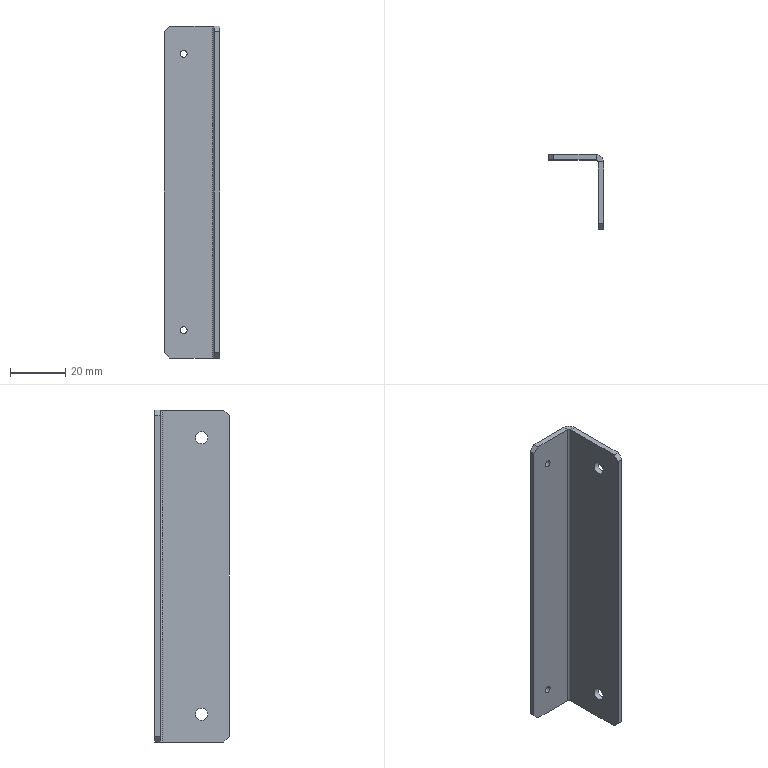Part | NX | 1 solid | 22 faces | box 20 x 27 x 120 mm | volume 10522 mm3 | plane 16 | cylinder 6 | commonest cylinder face diameters 2.5 x2 4.5 x2 1.473 x1 5.473 x1
STEP:
#1=CARTESIAN_POINT('',(-7.,0.,60.));
#2=VERTEX_POINT('',#1);
#3=CARTESIAN_POINT('',(8.263,0.,60.));
#4=VERTEX_POINT('',#3);
#5=CARTESIAN_POINT('',(-9.,0.,60.));
#6=DIRECTION('',(1.,0.,0.));
#7=VECTOR('',#6,1000.);
#8=LINE('',#5,#7);
#9=EDGE_CURVE('',#2,#4,#8,.T.);
#10=ORIENTED_EDGE('',*,*,#9,.F.);
#11=CARTESIAN_POINT('',(-7.,-2.,60.));
#12=VERTEX_POINT('',#11);
#13=CARTESIAN_POINT('',(-7.,-2.,60.));
#14=DIRECTION('',(0.,-1.,0.));
#15=VECTOR('',#14,1000.);
#16=LINE('',#13,#15);
#17=EDGE_CURVE('',#2,#12,#16,.T.);
#18=ORIENTED_EDGE('',*,*,#17,.T.);
#19=CARTESIAN_POINT('',(8.263,-2.,60.));
#20=VERTEX_POINT('',#19);
#21=CARTESIAN_POINT('',(-9.,-2.,60.));
#22=DIRECTION('',(1.,0.,0.));
#23=VECTOR('',#22,1000.);
#24=LINE('',#21,#23);
#25=EDGE_CURVE('',#12,#20,#24,.T.);
#26=ORIENTED_EDGE('',*,*,#25,.T.);
#27=CARTESIAN_POINT('',(8.263,-2.,60.));
#28=DIRECTION('',(0.,1.,0.));
#29=VECTOR('',#28,1000.);
#30=LINE('',#27,#29);
#31=EDGE_CURVE('',#20,#4,#30,.T.);
#32=ORIENTED_EDGE('',*,*,#31,.T.);
#33=EDGE_LOOP('',(#10,#18,#26,#32));
#34=FACE_BOUND('',#33,.T.);
#35=CARTESIAN_POINT('',(-9.,-2.,60.));
#36=DIRECTION('',(0.,0.,1.));
#37=DIRECTION('',(1.,0.,0.));
#38=AXIS2_PLACEMENT_3D('',#35,#36,#37);
#39=PLANE('',#38);
#40=ADVANCED_FACE('',(#34),#39,.T.);
#41=CARTESIAN_POINT('',(-2.,-2.,-51.25));
#42=VERTEX_POINT('',#41);
#43=CARTESIAN_POINT('',(-2.,-2.,-50.));
#44=DIRECTION('',(0.,-1.,0.));
#45=DIRECTION('',(0.,0.,-1.));
#46=AXIS2_PLACEMENT_3D('',#43,#44,#45);
#47=CIRCLE('',#46,1.25);
#48=EDGE_CURVE('',#42,#42,#47,.T.);
#49=ORIENTED_EDGE('',*,*,#48,.F.);
#50=EDGE_LOOP('',(#49));
#51=FACE_BOUND('',#50,.T.);
#52=CARTESIAN_POINT('',(-2.,-2.,48.75));
#53=VERTEX_POINT('',#52);
#54=CARTESIAN_POINT('',(-2.,-2.,50.));
#55=DIRECTION('',(0.,-1.,0.));
#56=DIRECTION('',(0.,0.,-1.));
#57=AXIS2_PLACEMENT_3D('',#54,#55,#56);
#58=CIRCLE('',#57,1.25);
#59=EDGE_CURVE('',#53,#53,#58,.T.);
#60=ORIENTED_EDGE('',*,*,#59,.F.);
#61=EDGE_LOOP('',(#60));
#62=FACE_BOUND('',#61,.T.);
#63=ORIENTED_EDGE('',*,*,#25,.F.);
#64=CARTESIAN_POINT('',(-9.,-2.,58.));
#65=VERTEX_POINT('',#64);
#66=CARTESIAN_POINT('',(-33.5,-2.,33.5));
#67=DIRECTION('',(0.7071,0.,0.7071));
#68=VECTOR('',#67,1000.);
#69=LINE('',#66,#68);
#70=EDGE_CURVE('',#12,#65,#69,.F.);
#71=ORIENTED_EDGE('',*,*,#70,.T.);
#72=CARTESIAN_POINT('',(-9.,-2.,-58.));
#73=VERTEX_POINT('',#72);
#74=CARTESIAN_POINT('',(-9.,-2.,60.));
#75=DIRECTION('',(0.,0.,1.));
#76=VECTOR('',#75,1000.);
#77=LINE('',#74,#76);
#78=EDGE_CURVE('',#73,#65,#77,.T.);
#79=ORIENTED_EDGE('',*,*,#78,.F.);
#80=CARTESIAN_POINT('',(-7.,-2.,-60.));
#81=VERTEX_POINT('',#80);
#82=CARTESIAN_POINT('',(-33.5,-2.,-33.5));
#83=DIRECTION('',(-0.7071,0.,0.7071));
#84=VECTOR('',#83,1000.);
#85=LINE('',#82,#84);
#86=EDGE_CURVE('',#73,#81,#85,.F.);
#87=ORIENTED_EDGE('',*,*,#86,.T.);
#88=CARTESIAN_POINT('',(8.263,-2.,-60.));
#89=VERTEX_POINT('',#88);
#90=CARTESIAN_POINT('',(-9.,-2.,-60.));
#91=DIRECTION('',(-1.,0.,0.));
#92=VECTOR('',#91,1000.);
#93=LINE('',#90,#92);
#94=EDGE_CURVE('',#89,#81,#93,.T.);
#95=ORIENTED_EDGE('',*,*,#94,.F.);
#96=CARTESIAN_POINT('',(8.263,-2.,60.));
#97=DIRECTION('',(0.,0.,1.));
#98=VECTOR('',#97,1000.);
#99=LINE('',#96,#98);
#100=EDGE_CURVE('',#20,#89,#99,.F.);
#101=ORIENTED_EDGE('',*,*,#100,.F.);
#102=EDGE_LOOP('',(#63,#71,#79,#87,#95,#101));
#103=FACE_BOUND('',#102,.T.);
#104=CARTESIAN_POINT('',(0.,-2.,0.));
#105=DIRECTION('',(0.,-1.,0.));
#106=DIRECTION('',(0.,0.,-1.));
#107=AXIS2_PLACEMENT_3D('',#104,#105,#106);
#108=PLANE('',#107);
#109=ADVANCED_FACE('',(#51,#62,#103),#108,.T.);
#110=CARTESIAN_POINT('',(-2.,0.,-48.75));
#111=VERTEX_POINT('',#110);
#112=CARTESIAN_POINT('',(-2.,0.,-50.));
#113=DIRECTION('',(0.,1.,0.));
#114=DIRECTION('',(0.,0.,1.));
#115=AXIS2_PLACEMENT_3D('',#112,#113,#114);
#116=CIRCLE('',#115,1.25);
#117=EDGE_CURVE('',#111,#111,#116,.T.);
#118=ORIENTED_EDGE('',*,*,#117,.F.);
#119=EDGE_LOOP('',(#118));
#120=FACE_BOUND('',#119,.T.);
#121=CARTESIAN_POINT('',(-2.,0.,51.25));
#122=VERTEX_POINT('',#121);
#123=CARTESIAN_POINT('',(-2.,0.,50.));
#124=DIRECTION('',(0.,1.,0.));
#125=DIRECTION('',(0.,0.,1.));
#126=AXIS2_PLACEMENT_3D('',#123,#124,#125);
#127=CIRCLE('',#126,1.25);
#128=EDGE_CURVE('',#122,#122,#127,.T.);
#129=ORIENTED_EDGE('',*,*,#128,.F.);
#130=EDGE_LOOP('',(#129));
#131=FACE_BOUND('',#130,.T.);
#132=CARTESIAN_POINT('',(-9.,0.,-58.));
#133=VERTEX_POINT('',#132);
#134=CARTESIAN_POINT('',(-9.,0.,58.));
#135=VERTEX_POINT('',#134);
#136=CARTESIAN_POINT('',(-9.,0.,60.));
#137=DIRECTION('',(0.,0.,1.));
#138=VECTOR('',#137,1000.);
#139=LINE('',#136,#138);
#140=EDGE_CURVE('',#133,#135,#139,.T.);
#141=ORIENTED_EDGE('',*,*,#140,.T.);
#142=CARTESIAN_POINT('',(-9.,0.,58.));
#143=DIRECTION('',(-0.7071,0.,-0.7071));
#144=VECTOR('',#143,1000.);
#145=LINE('',#142,#144);
#146=EDGE_CURVE('',#135,#2,#145,.F.);
#147=ORIENTED_EDGE('',*,*,#146,.T.);
#148=ORIENTED_EDGE('',*,*,#9,.T.);
#149=CARTESIAN_POINT('',(8.263,0.,-60.));
#150=VERTEX_POINT('',#149);
#151=CARTESIAN_POINT('',(8.263,0.,60.));
#152=DIRECTION('',(0.,0.,1.));
#153=VECTOR('',#152,1000.);
#154=LINE('',#151,#153);
#155=EDGE_CURVE('',#4,#150,#154,.F.);
#156=ORIENTED_EDGE('',*,*,#155,.T.);
#157=CARTESIAN_POINT('',(-7.,0.,-60.));
#158=VERTEX_POINT('',#157);
#159=CARTESIAN_POINT('',(-9.,0.,-60.));
#160=DIRECTION('',(-1.,0.,0.));
#161=VECTOR('',#160,1000.);
#162=LINE('',#159,#161);
#163=EDGE_CURVE('',#150,#158,#162,.T.);
#164=ORIENTED_EDGE('',*,*,#163,.T.);
#165=CARTESIAN_POINT('',(-7.,0.,-60.));
#166=DIRECTION('',(0.7071,0.,-0.7071));
#167=VECTOR('',#166,1000.);
#168=LINE('',#165,#167);
#169=EDGE_CURVE('',#158,#133,#168,.F.);
#170=ORIENTED_EDGE('',*,*,#169,.T.);
#171=EDGE_LOOP('',(#141,#147,#148,#156,#164,#170));
#172=FACE_BOUND('',#171,.T.);
#173=CARTESIAN_POINT('',(0.,0.,0.));
#174=DIRECTION('',(0.,-1.,0.));
#175=DIRECTION('',(0.,0.,-1.));
#176=AXIS2_PLACEMENT_3D('',#173,#174,#175);
#177=PLANE('',#176);
#178=ADVANCED_FACE('',(#120,#131,#172),#177,.F.);
#179=ORIENTED_EDGE('',*,*,#78,.T.);
#180=CARTESIAN_POINT('',(-9.,-2.,58.));
#181=DIRECTION('',(0.,1.,0.));
#182=VECTOR('',#181,1000.);
#183=LINE('',#180,#182);
#184=EDGE_CURVE('',#65,#135,#183,.T.);
#185=ORIENTED_EDGE('',*,*,#184,.T.);
#186=ORIENTED_EDGE('',*,*,#140,.F.);
#187=CARTESIAN_POINT('',(-9.,-2.,-58.));
#188=DIRECTION('',(0.,-1.,0.));
#189=VECTOR('',#188,1000.);
#190=LINE('',#187,#189);
#191=EDGE_CURVE('',#133,#73,#190,.T.);
#192=ORIENTED_EDGE('',*,*,#191,.T.);
#193=EDGE_LOOP('',(#179,#185,#186,#192));
#194=FACE_BOUND('',#193,.T.);
#195=CARTESIAN_POINT('',(-9.,-2.,60.));
#196=DIRECTION('',(-1.,0.,0.));
#197=DIRECTION('',(0.,0.,1.));
#198=AXIS2_PLACEMENT_3D('',#195,#196,#197);
#199=PLANE('',#198);
#200=ADVANCED_FACE('',(#194),#199,.T.);
#201=ORIENTED_EDGE('',*,*,#94,.T.);
#202=CARTESIAN_POINT('',(-7.,-2.,-60.));
#203=DIRECTION('',(0.,1.,0.));
#204=VECTOR('',#203,1000.);
#205=LINE('',#202,#204);
#206=EDGE_CURVE('',#81,#158,#205,.T.);
#207=ORIENTED_EDGE('',*,*,#206,.T.);
#208=ORIENTED_EDGE('',*,*,#163,.F.);
#209=CARTESIAN_POINT('',(8.263,-2.,-60.));
#210=DIRECTION('',(0.,1.,0.));
#211=VECTOR('',#210,1000.);
#212=LINE('',#209,#211);
#213=EDGE_CURVE('',#89,#150,#212,.T.);
#214=ORIENTED_EDGE('',*,*,#213,.F.);
#215=EDGE_LOOP('',(#201,#207,#208,#214));
#216=FACE_BOUND('',#215,.T.);
#217=CARTESIAN_POINT('',(-9.,-2.,-60.));
#218=DIRECTION('',(0.,0.,-1.));
#219=DIRECTION('',(-1.,0.,0.));
#220=AXIS2_PLACEMENT_3D('',#217,#218,#219);
#221=PLANE('',#220);
#222=ADVANCED_FACE('',(#216),#221,.T.);
#223=CARTESIAN_POINT('',(9.,-2.737,-60.));
#224=VERTEX_POINT('',#223);
#225=CARTESIAN_POINT('',(11.,-2.737,-60.));
#226=VERTEX_POINT('',#225);
#227=CARTESIAN_POINT('',(9.,-2.737,-60.));
#228=DIRECTION('',(1.,0.,0.));
#229=VECTOR('',#228,1000.);
#230=LINE('',#227,#229);
#231=EDGE_CURVE('',#224,#226,#230,.T.);
#232=ORIENTED_EDGE('',*,*,#231,.F.);
#233=CARTESIAN_POINT('',(8.263,-2.737,-60.));
#234=DIRECTION('',(0.,0.,1.));
#235=DIRECTION('',(1.,0.,0.));
#236=AXIS2_PLACEMENT_3D('',#233,#234,#235);
#237=CIRCLE('',#236,0.7366);
#238=EDGE_CURVE('',#89,#224,#237,.F.);
#239=ORIENTED_EDGE('',*,*,#238,.F.);
#240=ORIENTED_EDGE('',*,*,#213,.T.);
#241=CARTESIAN_POINT('',(8.263,-2.737,-60.));
#242=DIRECTION('',(0.,0.,1.));
#243=DIRECTION('',(1.,0.,0.));
#244=AXIS2_PLACEMENT_3D('',#241,#242,#243);
#245=CIRCLE('',#244,2.737);
#246=EDGE_CURVE('',#150,#226,#245,.F.);
#247=ORIENTED_EDGE('',*,*,#246,.T.);
#248=EDGE_LOOP('',(#232,#239,#240,#247));
#249=FACE_BOUND('',#248,.T.);
#250=CARTESIAN_POINT('',(8.263,-2.737,-60.));
#251=DIRECTION('',(0.,0.,-1.));
#252=DIRECTION('',(-1.,0.,0.));
#253=AXIS2_PLACEMENT_3D('',#250,#251,#252);
#254=PLANE('',#253);
#255=ADVANCED_FACE('',(#249),#254,.T.);
#256=CARTESIAN_POINT('',(9.,-2.737,60.));
#257=VERTEX_POINT('',#256);
#258=CARTESIAN_POINT('',(8.263,-2.737,60.));
#259=DIRECTION('',(0.,0.,1.));
#260=DIRECTION('',(1.,0.,0.));
#261=AXIS2_PLACEMENT_3D('',#258,#259,#260);
#262=CIRCLE('',#261,0.7366);
#263=EDGE_CURVE('',#257,#20,#262,.T.);
#264=ORIENTED_EDGE('',*,*,#263,.F.);
#265=CARTESIAN_POINT('',(11.,-2.737,60.));
#266=VERTEX_POINT('',#265);
#267=CARTESIAN_POINT('',(9.,-2.737,60.));
#268=DIRECTION('',(1.,0.,0.));
#269=VECTOR('',#268,1000.);
#270=LINE('',#267,#269);
#271=EDGE_CURVE('',#257,#266,#270,.T.);
#272=ORIENTED_EDGE('',*,*,#271,.T.);
#273=CARTESIAN_POINT('',(8.263,-2.737,60.));
#274=DIRECTION('',(0.,0.,1.));
#275=DIRECTION('',(1.,0.,0.));
#276=AXIS2_PLACEMENT_3D('',#273,#274,#275);
#277=CIRCLE('',#276,2.737);
#278=EDGE_CURVE('',#266,#4,#277,.T.);
#279=ORIENTED_EDGE('',*,*,#278,.T.);
#280=ORIENTED_EDGE('',*,*,#31,.F.);
#281=EDGE_LOOP('',(#264,#272,#279,#280));
#282=FACE_BOUND('',#281,.T.);
#283=CARTESIAN_POINT('',(8.263,-2.737,60.));
#284=DIRECTION('',(0.,0.,-1.));
#285=DIRECTION('',(-1.,0.,0.));
#286=AXIS2_PLACEMENT_3D('',#283,#284,#285);
#287=PLANE('',#286);
#288=ADVANCED_FACE('',(#282),#287,.F.);
#289=ORIENTED_EDGE('',*,*,#155,.F.);
#290=ORIENTED_EDGE('',*,*,#278,.F.);
#291=CARTESIAN_POINT('',(11.,-2.737,0.));
#292=DIRECTION('',(0.,0.,1.));
#293=VECTOR('',#292,1000.);
#294=LINE('',#291,#293);
#295=EDGE_CURVE('',#226,#266,#294,.T.);
#296=ORIENTED_EDGE('',*,*,#295,.F.);
#297=ORIENTED_EDGE('',*,*,#246,.F.);
#298=EDGE_LOOP('',(#289,#290,#296,#297));
#299=FACE_BOUND('',#298,.T.);
#300=CARTESIAN_POINT('',(8.263,-2.737,60.));
#301=DIRECTION('',(0.,0.,1.));
#302=DIRECTION('',(1.,0.,0.));
#303=AXIS2_PLACEMENT_3D('',#300,#301,#302);
#304=CYLINDRICAL_SURFACE('',#303,2.737);
#305=ADVANCED_FACE('',(#299),#304,.T.);
#306=ORIENTED_EDGE('',*,*,#100,.T.);
#307=ORIENTED_EDGE('',*,*,#238,.T.);
#308=CARTESIAN_POINT('',(9.,-2.737,-60.));
#309=DIRECTION('',(0.,0.,1.));
#310=VECTOR('',#309,1000.);
#311=LINE('',#308,#310);
#312=EDGE_CURVE('',#224,#257,#311,.T.);
#313=ORIENTED_EDGE('',*,*,#312,.T.);
#314=ORIENTED_EDGE('',*,*,#263,.T.);
#315=EDGE_LOOP('',(#306,#307,#313,#314));
#316=FACE_BOUND('',#315,.T.);
#317=CARTESIAN_POINT('',(8.263,-2.737,60.));
#318=DIRECTION('',(0.,0.,1.));
#319=DIRECTION('',(1.,0.,0.));
#320=AXIS2_PLACEMENT_3D('',#317,#318,#319);
#321=CYLINDRICAL_SURFACE('',#320,0.7366);
#322=ADVANCED_FACE('',(#316),#321,.F.);
#323=CARTESIAN_POINT('',(9.,-25.,60.));
#324=VERTEX_POINT('',#323);
#325=CARTESIAN_POINT('',(9.,-2.,60.));
#326=DIRECTION('',(0.,1.,0.));
#327=VECTOR('',#326,1000.);
#328=LINE('',#325,#327);
#329=EDGE_CURVE('',#324,#257,#328,.T.);
#330=ORIENTED_EDGE('',*,*,#329,.F.);
#331=CARTESIAN_POINT('',(11.,-25.,60.));
#332=VERTEX_POINT('',#331);
#333=CARTESIAN_POINT('',(11.,-25.,60.));
#334=DIRECTION('',(1.,0.,0.));
#335=VECTOR('',#334,1000.);
#336=LINE('',#333,#335);
#337=EDGE_CURVE('',#324,#332,#336,.T.);
#338=ORIENTED_EDGE('',*,*,#337,.T.);
#339=CARTESIAN_POINT('',(11.,-2.,60.));
#340=DIRECTION('',(0.,1.,0.));
#341=VECTOR('',#340,1000.);
#342=LINE('',#339,#341);
#343=EDGE_CURVE('',#332,#266,#342,.T.);
#344=ORIENTED_EDGE('',*,*,#343,.T.);
#345=ORIENTED_EDGE('',*,*,#271,.F.);
#346=EDGE_LOOP('',(#330,#338,#344,#345));
#347=FACE_BOUND('',#346,.T.);
#348=CARTESIAN_POINT('',(11.,-2.,60.));
#349=DIRECTION('',(0.,0.,1.));
#350=DIRECTION('',(1.,0.,0.));
#351=AXIS2_PLACEMENT_3D('',#348,#349,#350);
#352=PLANE('',#351);
#353=ADVANCED_FACE('',(#347),#352,.T.);
#354=CARTESIAN_POINT('',(11.,-25.,-60.));
#355=VERTEX_POINT('',#354);
#356=CARTESIAN_POINT('',(11.,-27.,-60.));
#357=DIRECTION('',(0.,-1.,0.));
#358=VECTOR('',#357,1000.);
#359=LINE('',#356,#358);
#360=EDGE_CURVE('',#226,#355,#359,.T.);
#361=ORIENTED_EDGE('',*,*,#360,.T.);
#362=CARTESIAN_POINT('',(9.,-25.,-60.));
#363=VERTEX_POINT('',#362);
#364=CARTESIAN_POINT('',(11.,-25.,-60.));
#365=DIRECTION('',(-1.,0.,0.));
#366=VECTOR('',#365,1000.);
#367=LINE('',#364,#366);
#368=EDGE_CURVE('',#355,#363,#367,.T.);
#369=ORIENTED_EDGE('',*,*,#368,.T.);
#370=CARTESIAN_POINT('',(9.,-27.,-60.));
#371=DIRECTION('',(0.,-1.,0.));
#372=VECTOR('',#371,1000.);
#373=LINE('',#370,#372);
#374=EDGE_CURVE('',#224,#363,#373,.T.);
#375=ORIENTED_EDGE('',*,*,#374,.F.);
#376=ORIENTED_EDGE('',*,*,#231,.T.);
#377=EDGE_LOOP('',(#361,#369,#375,#376));
#378=FACE_BOUND('',#377,.T.);
#379=CARTESIAN_POINT('',(11.,-27.,-60.));
#380=DIRECTION('',(0.,0.,-1.));
#381=DIRECTION('',(-1.,0.,0.));
#382=AXIS2_PLACEMENT_3D('',#379,#380,#381);
#383=PLANE('',#382);
#384=ADVANCED_FACE('',(#378),#383,.T.);
#385=CARTESIAN_POINT('',(11.,-17.,-47.75));
#386=VERTEX_POINT('',#385);
#387=CARTESIAN_POINT('',(11.,-17.,-50.));
#388=DIRECTION('',(-1.,0.,0.));
#389=DIRECTION('',(0.,0.,1.));
#390=AXIS2_PLACEMENT_3D('',#387,#388,#389);
#391=CIRCLE('',#390,2.25);
#392=EDGE_CURVE('',#386,#386,#391,.T.);
#393=ORIENTED_EDGE('',*,*,#392,.T.);
#394=EDGE_LOOP('',(#393));
#395=FACE_BOUND('',#394,.T.);
#396=CARTESIAN_POINT('',(11.,-17.,52.25));
#397=VERTEX_POINT('',#396);
#398=CARTESIAN_POINT('',(11.,-17.,50.));
#399=DIRECTION('',(-1.,0.,0.));
#400=DIRECTION('',(0.,0.,1.));
#401=AXIS2_PLACEMENT_3D('',#398,#399,#400);
#402=CIRCLE('',#401,2.25);
#403=EDGE_CURVE('',#397,#397,#402,.T.);
#404=ORIENTED_EDGE('',*,*,#403,.T.);
#405=EDGE_LOOP('',(#404));
#406=FACE_BOUND('',#405,.T.);
#407=CARTESIAN_POINT('',(11.,-27.,-58.));
#408=VERTEX_POINT('',#407);
#409=CARTESIAN_POINT('',(11.,-27.,58.));
#410=VERTEX_POINT('',#409);
#411=CARTESIAN_POINT('',(11.,-27.,60.));
#412=DIRECTION('',(0.,0.,1.));
#413=VECTOR('',#412,1000.);
#414=LINE('',#411,#413);
#415=EDGE_CURVE('',#408,#410,#414,.T.);
#416=ORIENTED_EDGE('',*,*,#415,.F.);
#417=CARTESIAN_POINT('',(11.,-42.5,-42.5));
#418=DIRECTION('',(0.,-0.7071,0.7071));
#419=VECTOR('',#418,1000.);
#420=LINE('',#417,#419);
#421=EDGE_CURVE('',#408,#355,#420,.F.);
#422=ORIENTED_EDGE('',*,*,#421,.T.);
#423=ORIENTED_EDGE('',*,*,#360,.F.);
#424=ORIENTED_EDGE('',*,*,#295,.T.);
#425=ORIENTED_EDGE('',*,*,#343,.F.);
#426=CARTESIAN_POINT('',(11.,-42.5,42.5));
#427=DIRECTION('',(0.,0.7071,0.7071));
#428=VECTOR('',#427,1000.);
#429=LINE('',#426,#428);
#430=EDGE_CURVE('',#332,#410,#429,.F.);
#431=ORIENTED_EDGE('',*,*,#430,.T.);
#432=EDGE_LOOP('',(#416,#422,#423,#424,#425,#431));
#433=FACE_BOUND('',#432,.T.);
#434=CARTESIAN_POINT('',(11.,0.,0.));
#435=DIRECTION('',(1.,0.,0.));
#436=DIRECTION('',(0.,1.,0.));
#437=AXIS2_PLACEMENT_3D('',#434,#435,#436);
#438=PLANE('',#437);
#439=ADVANCED_FACE('',(#395,#406,#433),#438,.T.);
#440=CARTESIAN_POINT('',(9.,-17.,-47.75));
#441=VERTEX_POINT('',#440);
#442=CARTESIAN_POINT('',(9.,-17.,-50.));
#443=DIRECTION('',(-1.,0.,0.));
#444=DIRECTION('',(0.,0.,1.));
#445=AXIS2_PLACEMENT_3D('',#442,#443,#444);
#446=CIRCLE('',#445,2.25);
#447=EDGE_CURVE('',#441,#441,#446,.T.);
#448=ORIENTED_EDGE('',*,*,#447,.F.);
#449=EDGE_LOOP('',(#448));
#450=FACE_BOUND('',#449,.T.);
#451=CARTESIAN_POINT('',(9.,-17.,52.25));
#452=VERTEX_POINT('',#451);
#453=CARTESIAN_POINT('',(9.,-17.,50.));
#454=DIRECTION('',(-1.,0.,0.));
#455=DIRECTION('',(0.,0.,1.));
#456=AXIS2_PLACEMENT_3D('',#453,#454,#455);
#457=CIRCLE('',#456,2.25);
#458=EDGE_CURVE('',#452,#452,#457,.T.);
#459=ORIENTED_EDGE('',*,*,#458,.F.);
#460=EDGE_LOOP('',(#459));
#461=FACE_BOUND('',#460,.T.);
#462=ORIENTED_EDGE('',*,*,#374,.T.);
#463=CARTESIAN_POINT('',(9.,-27.,-58.));
#464=VERTEX_POINT('',#463);
#465=CARTESIAN_POINT('',(9.,-25.,-60.));
#466=DIRECTION('',(0.,0.7071,-0.7071));
#467=VECTOR('',#466,1000.);
#468=LINE('',#465,#467);
#469=EDGE_CURVE('',#363,#464,#468,.F.);
#470=ORIENTED_EDGE('',*,*,#469,.T.);
#471=CARTESIAN_POINT('',(9.,-27.,58.));
#472=VERTEX_POINT('',#471);
#473=CARTESIAN_POINT('',(9.,-27.,60.));
#474=DIRECTION('',(0.,0.,1.));
#475=VECTOR('',#474,1000.);
#476=LINE('',#473,#475);
#477=EDGE_CURVE('',#464,#472,#476,.T.);
#478=ORIENTED_EDGE('',*,*,#477,.T.);
#479=CARTESIAN_POINT('',(9.,-27.,58.));
#480=DIRECTION('',(0.,-0.7071,-0.7071));
#481=VECTOR('',#480,1000.);
#482=LINE('',#479,#481);
#483=EDGE_CURVE('',#472,#324,#482,.F.);
#484=ORIENTED_EDGE('',*,*,#483,.T.);
#485=ORIENTED_EDGE('',*,*,#329,.T.);
#486=ORIENTED_EDGE('',*,*,#312,.F.);
#487=EDGE_LOOP('',(#462,#470,#478,#484,#485,#486));
#488=FACE_BOUND('',#487,.T.);
#489=CARTESIAN_POINT('',(9.,0.,0.));
#490=DIRECTION('',(1.,0.,0.));
#491=DIRECTION('',(0.,1.,0.));
#492=AXIS2_PLACEMENT_3D('',#489,#490,#491);
#493=PLANE('',#492);
#494=ADVANCED_FACE('',(#450,#461,#488),#493,.F.);
#495=ORIENTED_EDGE('',*,*,#477,.F.);
#496=CARTESIAN_POINT('',(11.,-27.,-58.));
#497=DIRECTION('',(1.,0.,0.));
#498=VECTOR('',#497,1000.);
#499=LINE('',#496,#498);
#500=EDGE_CURVE('',#464,#408,#499,.T.);
#501=ORIENTED_EDGE('',*,*,#500,.T.);
#502=ORIENTED_EDGE('',*,*,#415,.T.);
#503=CARTESIAN_POINT('',(11.,-27.,58.));
#504=DIRECTION('',(-1.,0.,0.));
#505=VECTOR('',#504,1000.);
#506=LINE('',#503,#505);
#507=EDGE_CURVE('',#410,#472,#506,.T.);
#508=ORIENTED_EDGE('',*,*,#507,.T.);
#509=EDGE_LOOP('',(#495,#501,#502,#508));
#510=FACE_BOUND('',#509,.T.);
#511=CARTESIAN_POINT('',(11.,-27.,60.));
#512=DIRECTION('',(0.,-1.,0.));
#513=DIRECTION('',(1.,0.,0.));
#514=AXIS2_PLACEMENT_3D('',#511,#512,#513);
#515=PLANE('',#514);
#516=ADVANCED_FACE('',(#510),#515,.T.);
#517=ORIENTED_EDGE('',*,*,#59,.T.);
#518=EDGE_LOOP('',(#517));
#519=FACE_BOUND('',#518,.T.);
#520=ORIENTED_EDGE('',*,*,#128,.T.);
#521=EDGE_LOOP('',(#520));
#522=FACE_BOUND('',#521,.T.);
#523=CARTESIAN_POINT('',(-2.,0.,50.));
#524=DIRECTION('',(0.,1.,0.));
#525=DIRECTION('',(0.,0.,1.));
#526=AXIS2_PLACEMENT_3D('',#523,#524,#525);
#527=CYLINDRICAL_SURFACE('',#526,1.25);
#528=ADVANCED_FACE('',(#519,#522),#527,.F.);
#529=ORIENTED_EDGE('',*,*,#48,.T.);
#530=EDGE_LOOP('',(#529));
#531=FACE_BOUND('',#530,.T.);
#532=ORIENTED_EDGE('',*,*,#117,.T.);
#533=EDGE_LOOP('',(#532));
#534=FACE_BOUND('',#533,.T.);
#535=CARTESIAN_POINT('',(-2.,0.,-50.));
#536=DIRECTION('',(0.,1.,0.));
#537=DIRECTION('',(0.,0.,1.));
#538=AXIS2_PLACEMENT_3D('',#535,#536,#537);
#539=CYLINDRICAL_SURFACE('',#538,1.25);
#540=ADVANCED_FACE('',(#531,#534),#539,.F.);
#541=ORIENTED_EDGE('',*,*,#403,.F.);
#542=EDGE_LOOP('',(#541));
#543=FACE_BOUND('',#542,.T.);
#544=ORIENTED_EDGE('',*,*,#458,.T.);
#545=EDGE_LOOP('',(#544));
#546=FACE_BOUND('',#545,.T.);
#547=CARTESIAN_POINT('',(9.,-17.,50.));
#548=DIRECTION('',(-1.,0.,0.));
#549=DIRECTION('',(0.,0.,1.));
#550=AXIS2_PLACEMENT_3D('',#547,#548,#549);
#551=CYLINDRICAL_SURFACE('',#550,2.25);
#552=ADVANCED_FACE('',(#543,#546),#551,.F.);
#553=ORIENTED_EDGE('',*,*,#392,.F.);
#554=EDGE_LOOP('',(#553));
#555=FACE_BOUND('',#554,.T.);
#556=ORIENTED_EDGE('',*,*,#447,.T.);
#557=EDGE_LOOP('',(#556));
#558=FACE_BOUND('',#557,.T.);
#559=CARTESIAN_POINT('',(9.,-17.,-50.));
#560=DIRECTION('',(-1.,0.,0.));
#561=DIRECTION('',(0.,0.,1.));
#562=AXIS2_PLACEMENT_3D('',#559,#560,#561);
#563=CYLINDRICAL_SURFACE('',#562,2.25);
#564=ADVANCED_FACE('',(#555,#558),#563,.F.);
#565=ORIENTED_EDGE('',*,*,#421,.F.);
#566=ORIENTED_EDGE('',*,*,#500,.F.);
#567=ORIENTED_EDGE('',*,*,#469,.F.);
#568=ORIENTED_EDGE('',*,*,#368,.F.);
#569=EDGE_LOOP('',(#565,#566,#567,#568));
#570=FACE_BOUND('',#569,.T.);
#571=CARTESIAN_POINT('',(11.,-25.,-60.));
#572=DIRECTION('',(0.,0.7071,0.7071));
#573=DIRECTION('',(-1.,0.,0.));
#574=AXIS2_PLACEMENT_3D('',#571,#572,#573);
#575=PLANE('',#574);
#576=ADVANCED_FACE('',(#570),#575,.F.);
#577=ORIENTED_EDGE('',*,*,#430,.F.);
#578=ORIENTED_EDGE('',*,*,#337,.F.);
#579=ORIENTED_EDGE('',*,*,#483,.F.);
#580=ORIENTED_EDGE('',*,*,#507,.F.);
#581=EDGE_LOOP('',(#577,#578,#579,#580));
#582=FACE_BOUND('',#581,.T.);
#583=CARTESIAN_POINT('',(11.,-27.,58.));
#584=DIRECTION('',(0.,0.7071,-0.7071));
#585=DIRECTION('',(-1.,0.,0.));
#586=AXIS2_PLACEMENT_3D('',#583,#584,#585);
#587=PLANE('',#586);
#588=ADVANCED_FACE('',(#582),#587,.F.);
#589=ORIENTED_EDGE('',*,*,#70,.F.);
#590=ORIENTED_EDGE('',*,*,#17,.F.);
#591=ORIENTED_EDGE('',*,*,#146,.F.);
#592=ORIENTED_EDGE('',*,*,#184,.F.);
#593=EDGE_LOOP('',(#589,#590,#591,#592));
#594=FACE_BOUND('',#593,.T.);
#595=CARTESIAN_POINT('',(-9.,-2.,58.));
#596=DIRECTION('',(0.7071,0.,-0.7071));
#597=DIRECTION('',(0.,1.,0.));
#598=AXIS2_PLACEMENT_3D('',#595,#596,#597);
#599=PLANE('',#598);
#600=ADVANCED_FACE('',(#594),#599,.F.);
#601=ORIENTED_EDGE('',*,*,#86,.F.);
#602=ORIENTED_EDGE('',*,*,#191,.F.);
#603=ORIENTED_EDGE('',*,*,#169,.F.);
#604=ORIENTED_EDGE('',*,*,#206,.F.);
#605=EDGE_LOOP('',(#601,#602,#603,#604));
#606=FACE_BOUND('',#605,.T.);
#607=CARTESIAN_POINT('',(-7.,-2.,-60.));
#608=DIRECTION('',(0.7071,0.,0.7071));
#609=DIRECTION('',(0.,1.,0.));
#610=AXIS2_PLACEMENT_3D('',#607,#608,#609);
#611=PLANE('',#610);
#612=ADVANCED_FACE('',(#606),#611,.F.);
#613=CLOSED_SHELL('',(#40,#109,#178,#200,#222,#255,#288,#305,#322,#353,#384,#439,#494,#516,#528,#540,#552,#564,#576,#588,#600,#612));
#614=MANIFOLD_SOLID_BREP('',#613);
#615=(LENGTH_UNIT()NAMED_UNIT(*)SI_UNIT(.MILLI.,.METRE.));
#616=UNCERTAINTY_MEASURE_WITH_UNIT(LENGTH_MEASURE(0.00001),#615,'','');
#617=(NAMED_UNIT(*)PLANE_ANGLE_UNIT()SI_UNIT($,.RADIAN.));
#618=(NAMED_UNIT(*)SI_UNIT($,.STERADIAN.)SOLID_ANGLE_UNIT());
#619=(GEOMETRIC_REPRESENTATION_CONTEXT(3)GLOBAL_UNCERTAINTY_ASSIGNED_CONTEXT((#616))GLOBAL_UNIT_ASSIGNED_CONTEXT((#615,#617,#618))REPRESENTATION_CONTEXT('',''));
#620=ADVANCED_BREP_SHAPE_REPRESENTATION('',(#614),#619);